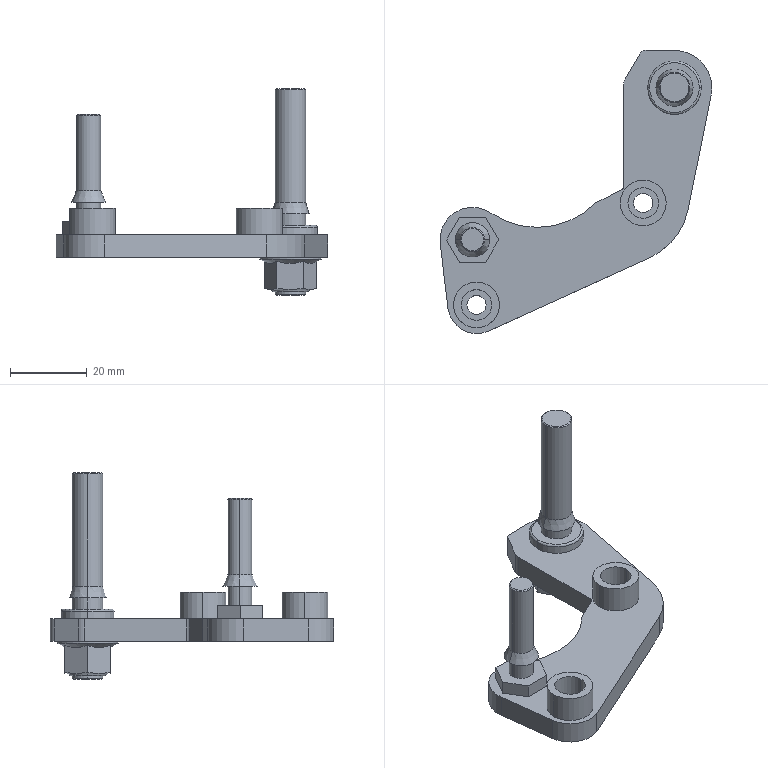Part | SolidWorks | features BaseBody 3 | 3 solids | 92 faces | box 70.95 x 73.951 x 54 mm | volume 17810 mm3 | cylinder 39 | plane 35 | cone 14 | torus 4 | commonest cylinder face diameters 8 x10 6.35 x6 5 x4 12 x4 6.351 x2 14 x2